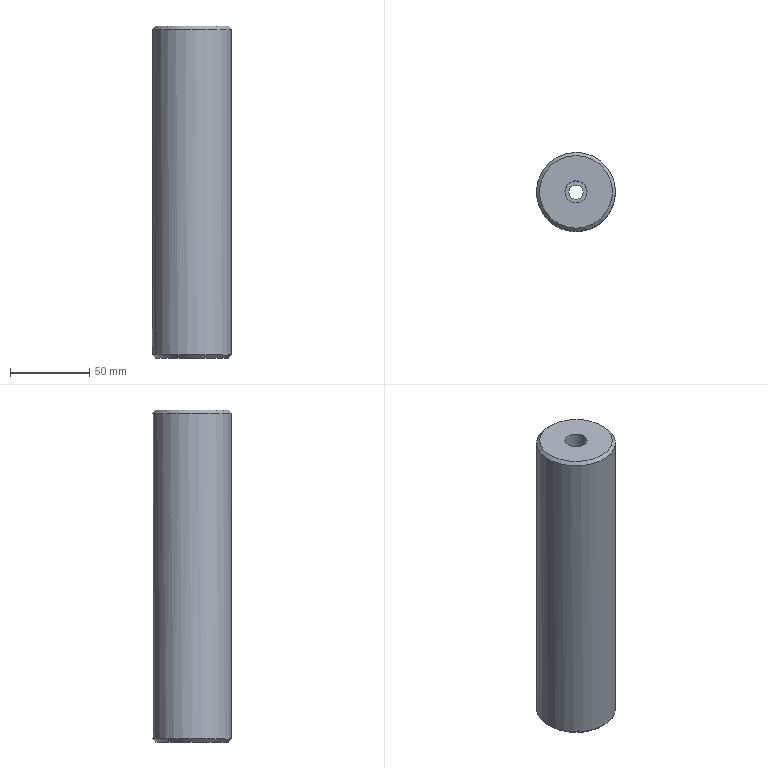Part | STEP file | MOLD-FOOT_id206_x_t | 1 solid | 8 faces | box 50 x 50 x 210 mm | volume 388518 mm3 | plane 3 | cylinder 3 | cone 2 | commonest cylinder face diameters 9 x1 14 x1 50 x1
STEP:
#1=CARTESIAN_POINT('',(134.5,145.5,376.));
#2=VERTEX_POINT('',#1);
#3=CARTESIAN_POINT('',(130.,145.5,376.));
#4=DIRECTION('',(0.,0.,-1.));
#5=DIRECTION('',(1.,0.,0.));
#6=AXIS2_PLACEMENT_3D('',#3,#4,#5);
#7=CIRCLE('',#6,4.5);
#8=EDGE_CURVE('',#2,#2,#7,.T.);
#9=ORIENTED_EDGE('',*,*,#8,.T.);
#10=EDGE_LOOP('',(#9));
#11=FACE_BOUND('',#10,.T.);
#12=CARTESIAN_POINT('',(137.,145.5,376.));
#13=VERTEX_POINT('',#12);
#14=CARTESIAN_POINT('',(130.,145.5,376.));
#15=DIRECTION('',(0.,0.,1.));
#16=DIRECTION('',(1.,0.,0.));
#17=AXIS2_PLACEMENT_3D('',#14,#15,#16);
#18=CIRCLE('',#17,7.);
#19=EDGE_CURVE('',#13,#13,#18,.T.);
#20=ORIENTED_EDGE('',*,*,#19,.T.);
#21=EDGE_LOOP('',(#20));
#22=FACE_BOUND('',#21,.T.);
#23=CARTESIAN_POINT('',(-80.,-60.,376.));
#24=DIRECTION('',(0.,0.,1.));
#25=DIRECTION('',(1.,0.,0.));
#26=AXIS2_PLACEMENT_3D('',#23,#24,#25);
#27=PLANE('',#26);
#28=ADVANCED_FACE('',(#11,#22),#27,.T.);
#29=ORIENTED_EDGE('',*,*,#19,.F.);
#30=EDGE_LOOP('',(#29));
#31=FACE_BOUND('',#30,.T.);
#32=CARTESIAN_POINT('',(137.,145.5,485.));
#33=VERTEX_POINT('',#32);
#34=CARTESIAN_POINT('',(130.,145.5,485.));
#35=DIRECTION('',(0.,0.,-1.));
#36=DIRECTION('',(1.,0.,0.));
#37=AXIS2_PLACEMENT_3D('',#34,#35,#36);
#38=CIRCLE('',#37,7.);
#39=EDGE_CURVE('',#33,#33,#38,.T.);
#40=ORIENTED_EDGE('',*,*,#39,.F.);
#41=EDGE_LOOP('',(#40));
#42=FACE_BOUND('',#41,.T.);
#43=CARTESIAN_POINT('',(130.,145.5,485.));
#44=DIRECTION('',(0.,0.,1.));
#45=DIRECTION('',(1.,0.,0.));
#46=AXIS2_PLACEMENT_3D('',#43,#44,#45);
#47=CYLINDRICAL_SURFACE('',#46,7.);
#48=ADVANCED_FACE('',(#31,#42),#47,.F.);
#49=CARTESIAN_POINT('',(134.5,145.5,275.));
#50=VERTEX_POINT('',#49);
#51=CARTESIAN_POINT('',(130.,145.5,275.));
#52=DIRECTION('',(0.,0.,-1.));
#53=DIRECTION('',(1.,0.,0.));
#54=AXIS2_PLACEMENT_3D('',#51,#52,#53);
#55=CIRCLE('',#54,4.5);
#56=EDGE_CURVE('',#50,#50,#55,.T.);
#57=ORIENTED_EDGE('',*,*,#56,.T.);
#58=EDGE_LOOP('',(#57));
#59=FACE_BOUND('',#58,.T.);
#60=ORIENTED_EDGE('',*,*,#8,.F.);
#61=EDGE_LOOP('',(#60));
#62=FACE_BOUND('',#61,.T.);
#63=CARTESIAN_POINT('',(130.,145.5,275.));
#64=DIRECTION('',(0.,0.,1.));
#65=DIRECTION('',(1.,0.,0.));
#66=AXIS2_PLACEMENT_3D('',#63,#64,#65);
#67=CYLINDRICAL_SURFACE('',#66,4.5);
#68=ADVANCED_FACE('',(#59,#62),#67,.F.);
#69=ORIENTED_EDGE('',*,*,#39,.T.);
#70=EDGE_LOOP('',(#69));
#71=FACE_BOUND('',#70,.T.);
#72=CARTESIAN_POINT('',(130.,168.5,485.));
#73=VERTEX_POINT('',#72);
#74=CARTESIAN_POINT('',(130.,145.5,485.));
#75=DIRECTION('',(0.,0.,-1.));
#76=DIRECTION('',(0.,1.,0.));
#77=AXIS2_PLACEMENT_3D('',#74,#75,#76);
#78=CIRCLE('',#77,23.);
#79=EDGE_CURVE('',#73,#73,#78,.T.);
#80=ORIENTED_EDGE('',*,*,#79,.F.);
#81=EDGE_LOOP('',(#80));
#82=FACE_BOUND('',#81,.T.);
#83=CARTESIAN_POINT('',(-80.,-60.,485.));
#84=DIRECTION('',(0.,0.,1.));
#85=DIRECTION('',(1.,0.,0.));
#86=AXIS2_PLACEMENT_3D('',#83,#84,#85);
#87=PLANE('',#86);
#88=ADVANCED_FACE('',(#71,#82),#87,.T.);
#89=ORIENTED_EDGE('',*,*,#56,.F.);
#90=EDGE_LOOP('',(#89));
#91=FACE_BOUND('',#90,.T.);
#92=CARTESIAN_POINT('',(153.,145.5,275.));
#93=VERTEX_POINT('',#92);
#94=CARTESIAN_POINT('',(130.,145.5,275.));
#95=DIRECTION('',(0.,0.,1.));
#96=DIRECTION('',(1.,0.,0.));
#97=AXIS2_PLACEMENT_3D('',#94,#95,#96);
#98=CIRCLE('',#97,23.);
#99=EDGE_CURVE('',#93,#93,#98,.T.);
#100=ORIENTED_EDGE('',*,*,#99,.F.);
#101=EDGE_LOOP('',(#100));
#102=FACE_BOUND('',#101,.T.);
#103=CARTESIAN_POINT('',(-80.,-60.,275.));
#104=DIRECTION('',(0.,0.,1.));
#105=DIRECTION('',(1.,0.,0.));
#106=AXIS2_PLACEMENT_3D('',#103,#104,#105);
#107=PLANE('',#106);
#108=ADVANCED_FACE('',(#91,#102),#107,.F.);
#109=CARTESIAN_POINT('',(155.,145.5,483.));
#110=VERTEX_POINT('',#109);
#111=CARTESIAN_POINT('',(130.,145.5,483.));
#112=DIRECTION('',(0.,0.,-1.));
#113=DIRECTION('',(1.,0.,0.));
#114=AXIS2_PLACEMENT_3D('',#111,#112,#113);
#115=CIRCLE('',#114,25.);
#116=EDGE_CURVE('',#110,#110,#115,.T.);
#117=ORIENTED_EDGE('',*,*,#116,.F.);
#118=EDGE_LOOP('',(#117));
#119=FACE_BOUND('',#118,.T.);
#120=ORIENTED_EDGE('',*,*,#79,.T.);
#121=EDGE_LOOP('',(#120));
#122=FACE_BOUND('',#121,.T.);
#123=CARTESIAN_POINT('',(130.,145.5,483.));
#124=DIRECTION('',(0.,0.,-1.));
#125=DIRECTION('',(0.,1.,0.));
#126=AXIS2_PLACEMENT_3D('',#123,#124,#125);
#127=CONICAL_SURFACE('',#126,25.,45.);
#128=ADVANCED_FACE('',(#119,#122),#127,.T.);
#129=CARTESIAN_POINT('',(155.,145.5,277.));
#130=VERTEX_POINT('',#129);
#131=CARTESIAN_POINT('',(130.,145.5,277.));
#132=DIRECTION('',(0.,0.,1.));
#133=DIRECTION('',(1.,0.,0.));
#134=AXIS2_PLACEMENT_3D('',#131,#132,#133);
#135=CIRCLE('',#134,25.);
#136=EDGE_CURVE('',#130,#130,#135,.T.);
#137=ORIENTED_EDGE('',*,*,#136,.F.);
#138=EDGE_LOOP('',(#137));
#139=FACE_BOUND('',#138,.T.);
#140=ORIENTED_EDGE('',*,*,#99,.T.);
#141=EDGE_LOOP('',(#140));
#142=FACE_BOUND('',#141,.T.);
#143=CARTESIAN_POINT('',(130.,145.5,277.));
#144=DIRECTION('',(0.,0.,1.));
#145=DIRECTION('',(1.,0.,0.));
#146=AXIS2_PLACEMENT_3D('',#143,#144,#145);
#147=CONICAL_SURFACE('',#146,25.,45.);
#148=ADVANCED_FACE('',(#139,#142),#147,.T.);
#149=ORIENTED_EDGE('',*,*,#116,.T.);
#150=EDGE_LOOP('',(#149));
#151=FACE_BOUND('',#150,.T.);
#152=ORIENTED_EDGE('',*,*,#136,.T.);
#153=EDGE_LOOP('',(#152));
#154=FACE_BOUND('',#153,.T.);
#155=CARTESIAN_POINT('',(130.,145.5,275.));
#156=DIRECTION('',(0.,0.,1.));
#157=DIRECTION('',(1.,0.,0.));
#158=AXIS2_PLACEMENT_3D('',#155,#156,#157);
#159=CYLINDRICAL_SURFACE('',#158,25.);
#160=ADVANCED_FACE('',(#151,#154),#159,.T.);
#161=CLOSED_SHELL('',(#28,#48,#68,#88,#108,#128,#148,#160));
#162=MANIFOLD_SOLID_BREP('',#161);
#163=(LENGTH_UNIT()NAMED_UNIT(*)SI_UNIT(.MILLI.,.METRE.));
#164=UNCERTAINTY_MEASURE_WITH_UNIT(LENGTH_MEASURE(0.00002),#163,'','');
#165=(NAMED_UNIT(*)PLANE_ANGLE_UNIT()SI_UNIT($,.RADIAN.));
#166=PLANE_ANGLE_MEASURE_WITH_UNIT(PLANE_ANGLE_MEASURE(0.01745),#165);
#167=DIMENSIONAL_EXPONENTS(0.,0.,0.,0.,0.,0.,0.);
#168=(CONVERSION_BASED_UNIT('DEGREE',#166)NAMED_UNIT(#167)PLANE_ANGLE_UNIT());
#169=(NAMED_UNIT(*)SI_UNIT($,.STERADIAN.)SOLID_ANGLE_UNIT());
#170=(GEOMETRIC_REPRESENTATION_CONTEXT(3)GLOBAL_UNCERTAINTY_ASSIGNED_CONTEXT((#164))GLOBAL_UNIT_ASSIGNED_CONTEXT((#163,#168,#169))REPRESENTATION_CONTEXT('',''));
#171=ADVANCED_BREP_SHAPE_REPRESENTATION('',(#162),#170);